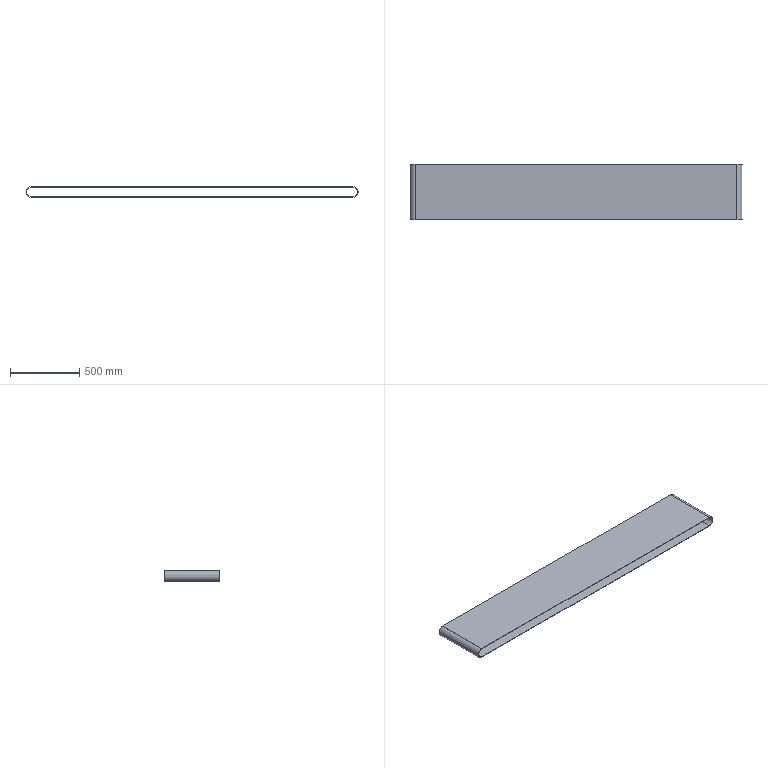Part | STEP file | 1.6米Belt | 1 solid | 10 faces | box 2391 x 398 x 76 mm | volume 5802047 mm3 | plane 6 | cylinder 4 | commonest cylinder face diameters 70 x2 76 x2
STEP:
#1=CARTESIAN_POINT('',(0.,398.,-38.));
#2=VERTEX_POINT('',#1);
#3=CARTESIAN_POINT('',(0.,398.,38.));
#4=VERTEX_POINT('',#3);
#5=CARTESIAN_POINT('',(0.,398.,0.));
#6=DIRECTION('',(0.,1.,0.));
#7=DIRECTION('',(0.,0.,1.));
#8=AXIS2_PLACEMENT_3D('',#5,#6,#7);
#9=CIRCLE('',#8,38.);
#10=EDGE_CURVE('',#2,#4,#9,.T.);
#11=ORIENTED_EDGE('',*,*,#10,.T.);
#12=CARTESIAN_POINT('',(2315.,398.,38.));
#13=VERTEX_POINT('',#12);
#14=CARTESIAN_POINT('',(0.,398.,38.));
#15=DIRECTION('',(1.,0.,0.));
#16=VECTOR('',#15,1000.);
#17=LINE('',#14,#16);
#18=EDGE_CURVE('',#4,#13,#17,.T.);
#19=ORIENTED_EDGE('',*,*,#18,.T.);
#20=CARTESIAN_POINT('',(2315.,398.,-38.));
#21=VERTEX_POINT('',#20);
#22=CARTESIAN_POINT('',(2315.,398.,0.));
#23=DIRECTION('',(0.,1.,0.));
#24=DIRECTION('',(0.,0.,1.));
#25=AXIS2_PLACEMENT_3D('',#22,#23,#24);
#26=CIRCLE('',#25,38.);
#27=EDGE_CURVE('',#13,#21,#26,.T.);
#28=ORIENTED_EDGE('',*,*,#27,.T.);
#29=CARTESIAN_POINT('',(0.,398.,-38.));
#30=DIRECTION('',(-1.,0.,0.));
#31=VECTOR('',#30,1000.);
#32=LINE('',#29,#31);
#33=EDGE_CURVE('',#21,#2,#32,.T.);
#34=ORIENTED_EDGE('',*,*,#33,.T.);
#35=EDGE_LOOP('',(#11,#19,#28,#34));
#36=FACE_OUTER_BOUND('',#35,.T.);
#37=CARTESIAN_POINT('',(0.,398.,35.));
#38=VERTEX_POINT('',#37);
#39=CARTESIAN_POINT('',(2315.,398.,35.));
#40=VERTEX_POINT('',#39);
#41=CARTESIAN_POINT('',(0.,398.,35.));
#42=DIRECTION('',(1.,0.,0.));
#43=VECTOR('',#42,1000.);
#44=LINE('',#41,#43);
#45=EDGE_CURVE('',#38,#40,#44,.T.);
#46=ORIENTED_EDGE('',*,*,#45,.F.);
#47=CARTESIAN_POINT('',(0.,398.,-35.));
#48=VERTEX_POINT('',#47);
#49=CARTESIAN_POINT('',(0.,398.,0.));
#50=DIRECTION('',(0.,1.,0.));
#51=DIRECTION('',(0.,0.,1.));
#52=AXIS2_PLACEMENT_3D('',#49,#50,#51);
#53=CIRCLE('',#52,35.);
#54=EDGE_CURVE('',#48,#38,#53,.T.);
#55=ORIENTED_EDGE('',*,*,#54,.F.);
#56=CARTESIAN_POINT('',(2315.,398.,-35.));
#57=VERTEX_POINT('',#56);
#58=CARTESIAN_POINT('',(0.,398.,-35.));
#59=DIRECTION('',(-1.,0.,0.));
#60=VECTOR('',#59,1000.);
#61=LINE('',#58,#60);
#62=EDGE_CURVE('',#57,#48,#61,.T.);
#63=ORIENTED_EDGE('',*,*,#62,.F.);
#64=CARTESIAN_POINT('',(2315.,398.,0.));
#65=DIRECTION('',(0.,1.,0.));
#66=DIRECTION('',(0.,0.,1.));
#67=AXIS2_PLACEMENT_3D('',#64,#65,#66);
#68=CIRCLE('',#67,35.);
#69=EDGE_CURVE('',#40,#57,#68,.T.);
#70=ORIENTED_EDGE('',*,*,#69,.F.);
#71=EDGE_LOOP('',(#46,#55,#63,#70));
#72=FACE_BOUND('',#71,.T.);
#73=CARTESIAN_POINT('',(0.,398.,0.));
#74=DIRECTION('',(0.,1.,0.));
#75=DIRECTION('',(0.,0.,1.));
#76=AXIS2_PLACEMENT_3D('',#73,#74,#75);
#77=PLANE('',#76);
#78=ADVANCED_FACE('',(#36,#72),#77,.T.);
#79=CARTESIAN_POINT('',(0.,0.,-38.));
#80=VERTEX_POINT('',#79);
#81=CARTESIAN_POINT('',(0.,0.,38.));
#82=VERTEX_POINT('',#81);
#83=CARTESIAN_POINT('',(0.,0.,0.));
#84=DIRECTION('',(0.,1.,0.));
#85=DIRECTION('',(0.,0.,1.));
#86=AXIS2_PLACEMENT_3D('',#83,#84,#85);
#87=CIRCLE('',#86,38.);
#88=EDGE_CURVE('',#80,#82,#87,.T.);
#89=ORIENTED_EDGE('',*,*,#88,.F.);
#90=CARTESIAN_POINT('',(2315.,0.,-38.));
#91=VERTEX_POINT('',#90);
#92=CARTESIAN_POINT('',(0.,0.,-38.));
#93=DIRECTION('',(-1.,0.,0.));
#94=VECTOR('',#93,1000.);
#95=LINE('',#92,#94);
#96=EDGE_CURVE('',#91,#80,#95,.T.);
#97=ORIENTED_EDGE('',*,*,#96,.F.);
#98=CARTESIAN_POINT('',(2315.,0.,38.));
#99=VERTEX_POINT('',#98);
#100=CARTESIAN_POINT('',(2315.,0.,0.));
#101=DIRECTION('',(0.,1.,0.));
#102=DIRECTION('',(0.,0.,1.));
#103=AXIS2_PLACEMENT_3D('',#100,#101,#102);
#104=CIRCLE('',#103,38.);
#105=EDGE_CURVE('',#99,#91,#104,.T.);
#106=ORIENTED_EDGE('',*,*,#105,.F.);
#107=CARTESIAN_POINT('',(0.,0.,38.));
#108=DIRECTION('',(1.,0.,0.));
#109=VECTOR('',#108,1000.);
#110=LINE('',#107,#109);
#111=EDGE_CURVE('',#82,#99,#110,.T.);
#112=ORIENTED_EDGE('',*,*,#111,.F.);
#113=EDGE_LOOP('',(#89,#97,#106,#112));
#114=FACE_OUTER_BOUND('',#113,.T.);
#115=CARTESIAN_POINT('',(0.,0.,-35.));
#116=VERTEX_POINT('',#115);
#117=CARTESIAN_POINT('',(0.,0.,35.));
#118=VERTEX_POINT('',#117);
#119=CARTESIAN_POINT('',(0.,0.,0.));
#120=DIRECTION('',(0.,1.,0.));
#121=DIRECTION('',(0.,0.,1.));
#122=AXIS2_PLACEMENT_3D('',#119,#120,#121);
#123=CIRCLE('',#122,35.);
#124=EDGE_CURVE('',#116,#118,#123,.T.);
#125=ORIENTED_EDGE('',*,*,#124,.T.);
#126=CARTESIAN_POINT('',(2315.,0.,35.));
#127=VERTEX_POINT('',#126);
#128=CARTESIAN_POINT('',(0.,0.,35.));
#129=DIRECTION('',(1.,0.,0.));
#130=VECTOR('',#129,1000.);
#131=LINE('',#128,#130);
#132=EDGE_CURVE('',#118,#127,#131,.T.);
#133=ORIENTED_EDGE('',*,*,#132,.T.);
#134=CARTESIAN_POINT('',(2315.,0.,-35.));
#135=VERTEX_POINT('',#134);
#136=CARTESIAN_POINT('',(2315.,0.,0.));
#137=DIRECTION('',(0.,1.,0.));
#138=DIRECTION('',(0.,0.,1.));
#139=AXIS2_PLACEMENT_3D('',#136,#137,#138);
#140=CIRCLE('',#139,35.);
#141=EDGE_CURVE('',#127,#135,#140,.T.);
#142=ORIENTED_EDGE('',*,*,#141,.T.);
#143=CARTESIAN_POINT('',(0.,0.,-35.));
#144=DIRECTION('',(-1.,0.,0.));
#145=VECTOR('',#144,1000.);
#146=LINE('',#143,#145);
#147=EDGE_CURVE('',#135,#116,#146,.T.);
#148=ORIENTED_EDGE('',*,*,#147,.T.);
#149=EDGE_LOOP('',(#125,#133,#142,#148));
#150=FACE_BOUND('',#149,.T.);
#151=CARTESIAN_POINT('',(0.,0.,0.));
#152=DIRECTION('',(0.,1.,0.));
#153=DIRECTION('',(0.,0.,1.));
#154=AXIS2_PLACEMENT_3D('',#151,#152,#153);
#155=PLANE('',#154);
#156=ADVANCED_FACE('',(#114,#150),#155,.F.);
#157=ORIENTED_EDGE('',*,*,#88,.T.);
#158=CARTESIAN_POINT('',(0.,398.,38.));
#159=DIRECTION('',(0.,-1.,0.));
#160=VECTOR('',#159,1000.);
#161=LINE('',#158,#160);
#162=EDGE_CURVE('',#4,#82,#161,.T.);
#163=ORIENTED_EDGE('',*,*,#162,.F.);
#164=ORIENTED_EDGE('',*,*,#10,.F.);
#165=CARTESIAN_POINT('',(0.,398.,-38.));
#166=DIRECTION('',(0.,-1.,0.));
#167=VECTOR('',#166,1000.);
#168=LINE('',#165,#167);
#169=EDGE_CURVE('',#2,#80,#168,.T.);
#170=ORIENTED_EDGE('',*,*,#169,.T.);
#171=EDGE_LOOP('',(#157,#163,#164,#170));
#172=FACE_OUTER_BOUND('',#171,.T.);
#173=CARTESIAN_POINT('',(0.,398.,0.));
#174=DIRECTION('',(0.,-1.,0.));
#175=DIRECTION('',(0.,0.,-1.));
#176=AXIS2_PLACEMENT_3D('',#173,#174,#175);
#177=CYLINDRICAL_SURFACE('',#176,38.);
#178=ADVANCED_FACE('',(#172),#177,.T.);
#179=ORIENTED_EDGE('',*,*,#111,.T.);
#180=CARTESIAN_POINT('',(2315.,398.,38.));
#181=DIRECTION('',(0.,-1.,0.));
#182=VECTOR('',#181,1000.);
#183=LINE('',#180,#182);
#184=EDGE_CURVE('',#13,#99,#183,.T.);
#185=ORIENTED_EDGE('',*,*,#184,.F.);
#186=ORIENTED_EDGE('',*,*,#18,.F.);
#187=ORIENTED_EDGE('',*,*,#162,.T.);
#188=EDGE_LOOP('',(#179,#185,#186,#187));
#189=FACE_OUTER_BOUND('',#188,.T.);
#190=CARTESIAN_POINT('',(0.,398.,38.));
#191=DIRECTION('',(0.,0.,-1.));
#192=DIRECTION('',(-1.,0.,0.));
#193=AXIS2_PLACEMENT_3D('',#190,#191,#192);
#194=PLANE('',#193);
#195=ADVANCED_FACE('',(#189),#194,.F.);
#196=ORIENTED_EDGE('',*,*,#105,.T.);
#197=CARTESIAN_POINT('',(2315.,398.,-38.));
#198=DIRECTION('',(0.,-1.,0.));
#199=VECTOR('',#198,1000.);
#200=LINE('',#197,#199);
#201=EDGE_CURVE('',#21,#91,#200,.T.);
#202=ORIENTED_EDGE('',*,*,#201,.F.);
#203=ORIENTED_EDGE('',*,*,#27,.F.);
#204=ORIENTED_EDGE('',*,*,#184,.T.);
#205=EDGE_LOOP('',(#196,#202,#203,#204));
#206=FACE_OUTER_BOUND('',#205,.T.);
#207=CARTESIAN_POINT('',(2315.,398.,0.));
#208=DIRECTION('',(0.,-1.,0.));
#209=DIRECTION('',(0.,0.,-1.));
#210=AXIS2_PLACEMENT_3D('',#207,#208,#209);
#211=CYLINDRICAL_SURFACE('',#210,38.);
#212=ADVANCED_FACE('',(#206),#211,.T.);
#213=ORIENTED_EDGE('',*,*,#96,.T.);
#214=ORIENTED_EDGE('',*,*,#169,.F.);
#215=ORIENTED_EDGE('',*,*,#33,.F.);
#216=ORIENTED_EDGE('',*,*,#201,.T.);
#217=EDGE_LOOP('',(#213,#214,#215,#216));
#218=FACE_OUTER_BOUND('',#217,.T.);
#219=CARTESIAN_POINT('',(0.,398.,-38.));
#220=DIRECTION('',(0.,0.,1.));
#221=DIRECTION('',(1.,0.,0.));
#222=AXIS2_PLACEMENT_3D('',#219,#220,#221);
#223=PLANE('',#222);
#224=ADVANCED_FACE('',(#218),#223,.F.);
#225=ORIENTED_EDGE('',*,*,#124,.F.);
#226=CARTESIAN_POINT('',(0.,398.,-35.));
#227=DIRECTION('',(0.,-1.,0.));
#228=VECTOR('',#227,1000.);
#229=LINE('',#226,#228);
#230=EDGE_CURVE('',#48,#116,#229,.T.);
#231=ORIENTED_EDGE('',*,*,#230,.F.);
#232=ORIENTED_EDGE('',*,*,#54,.T.);
#233=CARTESIAN_POINT('',(0.,398.,35.));
#234=DIRECTION('',(0.,-1.,0.));
#235=VECTOR('',#234,1000.);
#236=LINE('',#233,#235);
#237=EDGE_CURVE('',#38,#118,#236,.T.);
#238=ORIENTED_EDGE('',*,*,#237,.T.);
#239=EDGE_LOOP('',(#225,#231,#232,#238));
#240=FACE_OUTER_BOUND('',#239,.T.);
#241=CARTESIAN_POINT('',(0.,398.,0.));
#242=DIRECTION('',(0.,-1.,0.));
#243=DIRECTION('',(0.,0.,-1.));
#244=AXIS2_PLACEMENT_3D('',#241,#242,#243);
#245=CYLINDRICAL_SURFACE('',#244,35.);
#246=ADVANCED_FACE('',(#240),#245,.F.);
#247=ORIENTED_EDGE('',*,*,#132,.F.);
#248=ORIENTED_EDGE('',*,*,#237,.F.);
#249=ORIENTED_EDGE('',*,*,#45,.T.);
#250=CARTESIAN_POINT('',(2315.,398.,35.));
#251=DIRECTION('',(0.,-1.,0.));
#252=VECTOR('',#251,1000.);
#253=LINE('',#250,#252);
#254=EDGE_CURVE('',#40,#127,#253,.T.);
#255=ORIENTED_EDGE('',*,*,#254,.T.);
#256=EDGE_LOOP('',(#247,#248,#249,#255));
#257=FACE_OUTER_BOUND('',#256,.T.);
#258=CARTESIAN_POINT('',(0.,398.,35.));
#259=DIRECTION('',(0.,0.,-1.));
#260=DIRECTION('',(-1.,0.,0.));
#261=AXIS2_PLACEMENT_3D('',#258,#259,#260);
#262=PLANE('',#261);
#263=ADVANCED_FACE('',(#257),#262,.T.);
#264=ORIENTED_EDGE('',*,*,#141,.F.);
#265=ORIENTED_EDGE('',*,*,#254,.F.);
#266=ORIENTED_EDGE('',*,*,#69,.T.);
#267=CARTESIAN_POINT('',(2315.,398.,-35.));
#268=DIRECTION('',(0.,-1.,0.));
#269=VECTOR('',#268,1000.);
#270=LINE('',#267,#269);
#271=EDGE_CURVE('',#57,#135,#270,.T.);
#272=ORIENTED_EDGE('',*,*,#271,.T.);
#273=EDGE_LOOP('',(#264,#265,#266,#272));
#274=FACE_OUTER_BOUND('',#273,.T.);
#275=CARTESIAN_POINT('',(2315.,398.,0.));
#276=DIRECTION('',(0.,-1.,0.));
#277=DIRECTION('',(0.,0.,-1.));
#278=AXIS2_PLACEMENT_3D('',#275,#276,#277);
#279=CYLINDRICAL_SURFACE('',#278,35.);
#280=ADVANCED_FACE('',(#274),#279,.F.);
#281=ORIENTED_EDGE('',*,*,#147,.F.);
#282=ORIENTED_EDGE('',*,*,#271,.F.);
#283=ORIENTED_EDGE('',*,*,#62,.T.);
#284=ORIENTED_EDGE('',*,*,#230,.T.);
#285=EDGE_LOOP('',(#281,#282,#283,#284));
#286=FACE_OUTER_BOUND('',#285,.T.);
#287=CARTESIAN_POINT('',(0.,398.,-35.));
#288=DIRECTION('',(0.,0.,1.));
#289=DIRECTION('',(1.,0.,0.));
#290=AXIS2_PLACEMENT_3D('',#287,#288,#289);
#291=PLANE('',#290);
#292=ADVANCED_FACE('',(#286),#291,.T.);
#293=CLOSED_SHELL('',(#78,#156,#178,#195,#212,#224,#246,#263,#280,#292));
#294=MANIFOLD_SOLID_BREP('',#293);
#295=CARTESIAN_POINT('',(0.,0.,0.));
#296=DIRECTION('',(0.,0.,1.));
#297=DIRECTION('',(1.,0.,0.));
#298=AXIS2_PLACEMENT_3D('',#295,#296,#297);
#299=(LENGTH_UNIT()NAMED_UNIT(*)SI_UNIT(.MILLI.,.METRE.));
#300=UNCERTAINTY_MEASURE_WITH_UNIT(LENGTH_MEASURE(0.00001),#299,'','');
#301=(NAMED_UNIT(*)PLANE_ANGLE_UNIT()SI_UNIT($,.RADIAN.));
#302=(NAMED_UNIT(*)SI_UNIT($,.STERADIAN.)SOLID_ANGLE_UNIT());
#303=(GEOMETRIC_REPRESENTATION_CONTEXT(3)GLOBAL_UNCERTAINTY_ASSIGNED_CONTEXT((#300))GLOBAL_UNIT_ASSIGNED_CONTEXT((#299,#301,#302))REPRESENTATION_CONTEXT('',''));
#304=ADVANCED_BREP_SHAPE_REPRESENTATION('',(#294,#298),#303);